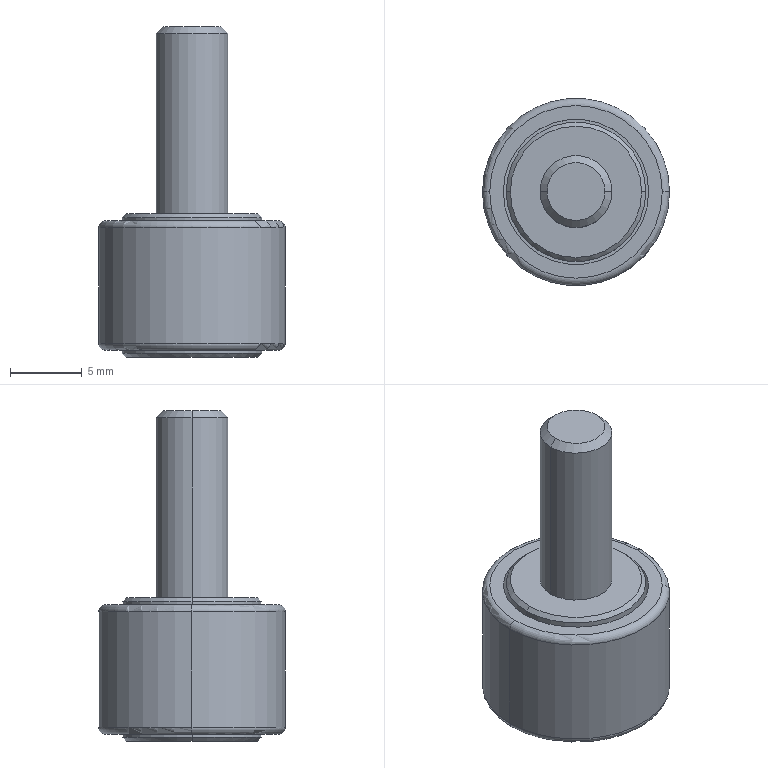Part | NX | features BREP 1 | 1 solid | 36 faces | box 13 x 13 x 23 mm | volume 1465 mm3 | plane 14 | cylinder 12 | cone 6 | torus 4 | commonest cylinder face diameters 9.7 x4 10.1 x4 5 x2 13 x2
STEP:
#1=CARTESIAN_POINT('',(4.567,0.,-23.));
#2=VERTEX_POINT('',#1);
#3=CARTESIAN_POINT('',(-4.567,0.,-23.));
#4=VERTEX_POINT('',#3);
#5=CARTESIAN_POINT('',(0.,0.,-23.));
#6=DIRECTION('',(0.,0.,1.));
#7=DIRECTION('',(1.,0.,0.));
#8=AXIS2_PLACEMENT_3D('',#5,#6,#7);
#9=CIRCLE('',#8,4.567);
#10=EDGE_CURVE('',#2,#4,#9,.T.);
#11=ORIENTED_EDGE('',*,*,#10,.T.);
#12=CARTESIAN_POINT('',(-4.85,0.,-22.717));
#13=VERTEX_POINT('',#12);
#14=CARTESIAN_POINT('',(-4.567,0.,-23.));
#15=DIRECTION('',(-0.7071,0.,0.7071));
#16=VECTOR('',#15,1000.);
#17=LINE('',#14,#16);
#18=EDGE_CURVE('',#4,#13,#17,.T.);
#19=ORIENTED_EDGE('',*,*,#18,.T.);
#20=CARTESIAN_POINT('',(4.85,0.,-22.717));
#21=VERTEX_POINT('',#20);
#22=CARTESIAN_POINT('',(0.,0.,-22.717));
#23=DIRECTION('',(0.,0.,1.));
#24=DIRECTION('',(1.,0.,0.));
#25=AXIS2_PLACEMENT_3D('',#22,#23,#24);
#26=CIRCLE('',#25,4.85);
#27=EDGE_CURVE('',#21,#13,#26,.T.);
#28=ORIENTED_EDGE('',*,*,#27,.F.);
#29=CARTESIAN_POINT('',(4.567,0.,-23.));
#30=DIRECTION('',(0.7071,0.,0.7071));
#31=VECTOR('',#30,1000.);
#32=LINE('',#29,#31);
#33=EDGE_CURVE('',#2,#21,#32,.T.);
#34=ORIENTED_EDGE('',*,*,#33,.F.);
#35=EDGE_LOOP('',(#11,#19,#28,#34));
#36=FACE_BOUND('',#35,.T.);
#37=CARTESIAN_POINT('',(0.,0.,-23.));
#38=DIRECTION('',(0.,0.,1.));
#39=DIRECTION('',(-1.,0.,0.));
#40=AXIS2_PLACEMENT_3D('',#37,#38,#39);
#41=CONICAL_SURFACE('',#40,4.567,0.7854);
#42=ADVANCED_FACE('',(#36),#41,.T.);
#43=ORIENTED_EDGE('',*,*,#27,.T.);
#44=CARTESIAN_POINT('',(-4.85,0.,-21.));
#45=VERTEX_POINT('',#44);
#46=CARTESIAN_POINT('',(-4.85,0.,-23.));
#47=DIRECTION('',(0.,0.,1.));
#48=VECTOR('',#47,1000.);
#49=LINE('',#46,#48);
#50=EDGE_CURVE('',#13,#45,#49,.T.);
#51=ORIENTED_EDGE('',*,*,#50,.T.);
#52=CARTESIAN_POINT('',(4.85,0.,-21.));
#53=VERTEX_POINT('',#52);
#54=CARTESIAN_POINT('',(0.,0.,-21.));
#55=DIRECTION('',(0.,0.,1.));
#56=DIRECTION('',(1.,0.,0.));
#57=AXIS2_PLACEMENT_3D('',#54,#55,#56);
#58=CIRCLE('',#57,4.85);
#59=EDGE_CURVE('',#53,#45,#58,.T.);
#60=ORIENTED_EDGE('',*,*,#59,.F.);
#61=CARTESIAN_POINT('',(4.85,0.,-23.));
#62=DIRECTION('',(0.,0.,1.));
#63=VECTOR('',#62,1000.);
#64=LINE('',#61,#63);
#65=EDGE_CURVE('',#21,#53,#64,.T.);
#66=ORIENTED_EDGE('',*,*,#65,.F.);
#67=EDGE_LOOP('',(#43,#51,#60,#66));
#68=FACE_BOUND('',#67,.T.);
#69=CARTESIAN_POINT('',(0.,0.,-23.));
#70=DIRECTION('',(0.,0.,1.));
#71=DIRECTION('',(-1.,0.,0.));
#72=AXIS2_PLACEMENT_3D('',#69,#70,#71);
#73=CYLINDRICAL_SURFACE('',#72,4.85);
#74=ADVANCED_FACE('',(#68),#73,.T.);
#75=CARTESIAN_POINT('',(-5.05,0.,-22.5));
#76=VERTEX_POINT('',#75);
#77=CARTESIAN_POINT('',(5.05,0.,-22.5));
#78=VERTEX_POINT('',#77);
#79=CARTESIAN_POINT('',(0.,0.,-22.5));
#80=DIRECTION('',(0.,0.,1.));
#81=DIRECTION('',(1.,0.,0.));
#82=AXIS2_PLACEMENT_3D('',#79,#80,#81);
#83=CIRCLE('',#82,5.05);
#84=EDGE_CURVE('',#76,#78,#83,.T.);
#85=ORIENTED_EDGE('',*,*,#84,.F.);
#86=CARTESIAN_POINT('',(-5.05,0.,-21.));
#87=VERTEX_POINT('',#86);
#88=CARTESIAN_POINT('',(-5.05,0.,-23.));
#89=DIRECTION('',(0.,0.,1.));
#90=VECTOR('',#89,1000.);
#91=LINE('',#88,#90);
#92=EDGE_CURVE('',#76,#87,#91,.T.);
#93=ORIENTED_EDGE('',*,*,#92,.T.);
#94=CARTESIAN_POINT('',(5.05,0.,-21.));
#95=VERTEX_POINT('',#94);
#96=CARTESIAN_POINT('',(0.,0.,-21.));
#97=DIRECTION('',(0.,0.,1.));
#98=DIRECTION('',(1.,0.,0.));
#99=AXIS2_PLACEMENT_3D('',#96,#97,#98);
#100=CIRCLE('',#99,5.05);
#101=EDGE_CURVE('',#87,#95,#100,.T.);
#102=ORIENTED_EDGE('',*,*,#101,.T.);
#103=CARTESIAN_POINT('',(5.05,0.,-23.));
#104=DIRECTION('',(0.,0.,1.));
#105=VECTOR('',#104,1000.);
#106=LINE('',#103,#105);
#107=EDGE_CURVE('',#78,#95,#106,.T.);
#108=ORIENTED_EDGE('',*,*,#107,.F.);
#109=EDGE_LOOP('',(#85,#93,#102,#108));
#110=FACE_BOUND('',#109,.T.);
#111=CARTESIAN_POINT('',(0.,0.,-23.));
#112=DIRECTION('',(0.,0.,1.));
#113=DIRECTION('',(-1.,0.,0.));
#114=AXIS2_PLACEMENT_3D('',#111,#112,#113);
#115=CYLINDRICAL_SURFACE('',#114,5.05);
#116=ADVANCED_FACE('',(#110),#115,.F.);
#117=CARTESIAN_POINT('',(6.,0.,-22.5));
#118=VERTEX_POINT('',#117);
#119=CARTESIAN_POINT('',(-6.,0.,-22.5));
#120=VERTEX_POINT('',#119);
#121=CARTESIAN_POINT('',(0.,0.,-22.5));
#122=DIRECTION('',(0.,0.,1.));
#123=DIRECTION('',(1.,0.,0.));
#124=AXIS2_PLACEMENT_3D('',#121,#122,#123);
#125=CIRCLE('',#124,6.);
#126=EDGE_CURVE('',#118,#120,#125,.T.);
#127=ORIENTED_EDGE('',*,*,#126,.T.);
#128=CARTESIAN_POINT('',(-6.5,0.,-22.));
#129=VERTEX_POINT('',#128);
#130=CARTESIAN_POINT('',(-6.,0.,-22.));
#131=DIRECTION('',(0.,1.,0.));
#132=DIRECTION('',(-1.,0.,0.));
#133=AXIS2_PLACEMENT_3D('',#130,#131,#132);
#134=CIRCLE('',#133,0.5);
#135=EDGE_CURVE('',#120,#129,#134,.T.);
#136=ORIENTED_EDGE('',*,*,#135,.T.);
#137=CARTESIAN_POINT('',(6.5,0.,-22.));
#138=VERTEX_POINT('',#137);
#139=CARTESIAN_POINT('',(0.,0.,-22.));
#140=DIRECTION('',(0.,0.,1.));
#141=DIRECTION('',(1.,0.,0.));
#142=AXIS2_PLACEMENT_3D('',#139,#140,#141);
#143=CIRCLE('',#142,6.5);
#144=EDGE_CURVE('',#138,#129,#143,.T.);
#145=ORIENTED_EDGE('',*,*,#144,.F.);
#146=CARTESIAN_POINT('',(6.,0.,-22.));
#147=DIRECTION('',(0.,-1.,0.));
#148=DIRECTION('',(0.,0.,-1.));
#149=AXIS2_PLACEMENT_3D('',#146,#147,#148);
#150=CIRCLE('',#149,0.5);
#151=EDGE_CURVE('',#118,#138,#150,.T.);
#152=ORIENTED_EDGE('',*,*,#151,.F.);
#153=EDGE_LOOP('',(#127,#136,#145,#152));
#154=FACE_BOUND('',#153,.T.);
#155=CARTESIAN_POINT('',(0.,0.,-22.));
#156=DIRECTION('',(0.,0.,1.));
#157=DIRECTION('',(-1.,0.,0.));
#158=AXIS2_PLACEMENT_3D('',#155,#156,#157);
#159=TOROIDAL_SURFACE('',#158,6.,0.5);
#160=ADVANCED_FACE('',(#154),#159,.T.);
#161=ORIENTED_EDGE('',*,*,#144,.T.);
#162=CARTESIAN_POINT('',(-6.5,0.,-14.));
#163=VERTEX_POINT('',#162);
#164=CARTESIAN_POINT('',(-6.5,0.,-23.));
#165=DIRECTION('',(0.,0.,1.));
#166=VECTOR('',#165,1000.);
#167=LINE('',#164,#166);
#168=EDGE_CURVE('',#129,#163,#167,.T.);
#169=ORIENTED_EDGE('',*,*,#168,.T.);
#170=CARTESIAN_POINT('',(6.5,0.,-14.));
#171=VERTEX_POINT('',#170);
#172=CARTESIAN_POINT('',(0.,0.,-14.));
#173=DIRECTION('',(0.,0.,1.));
#174=DIRECTION('',(1.,0.,0.));
#175=AXIS2_PLACEMENT_3D('',#172,#173,#174);
#176=CIRCLE('',#175,6.5);
#177=EDGE_CURVE('',#171,#163,#176,.T.);
#178=ORIENTED_EDGE('',*,*,#177,.F.);
#179=CARTESIAN_POINT('',(6.5,0.,-23.));
#180=DIRECTION('',(0.,0.,1.));
#181=VECTOR('',#180,1000.);
#182=LINE('',#179,#181);
#183=EDGE_CURVE('',#138,#171,#182,.T.);
#184=ORIENTED_EDGE('',*,*,#183,.F.);
#185=EDGE_LOOP('',(#161,#169,#178,#184));
#186=FACE_BOUND('',#185,.T.);
#187=CARTESIAN_POINT('',(0.,0.,-23.));
#188=DIRECTION('',(0.,0.,1.));
#189=DIRECTION('',(-1.,0.,0.));
#190=AXIS2_PLACEMENT_3D('',#187,#188,#189);
#191=CYLINDRICAL_SURFACE('',#190,6.5);
#192=ADVANCED_FACE('',(#186),#191,.T.);
#193=ORIENTED_EDGE('',*,*,#177,.T.);
#194=CARTESIAN_POINT('',(-6.,0.,-13.5));
#195=VERTEX_POINT('',#194);
#196=CARTESIAN_POINT('',(-6.,0.,-14.));
#197=DIRECTION('',(0.,1.,0.));
#198=DIRECTION('',(-1.,0.,0.));
#199=AXIS2_PLACEMENT_3D('',#196,#197,#198);
#200=CIRCLE('',#199,0.5);
#201=EDGE_CURVE('',#163,#195,#200,.T.);
#202=ORIENTED_EDGE('',*,*,#201,.T.);
#203=CARTESIAN_POINT('',(6.,0.,-13.5));
#204=VERTEX_POINT('',#203);
#205=CARTESIAN_POINT('',(0.,0.,-13.5));
#206=DIRECTION('',(0.,0.,1.));
#207=DIRECTION('',(1.,0.,0.));
#208=AXIS2_PLACEMENT_3D('',#205,#206,#207);
#209=CIRCLE('',#208,6.);
#210=EDGE_CURVE('',#204,#195,#209,.T.);
#211=ORIENTED_EDGE('',*,*,#210,.F.);
#212=CARTESIAN_POINT('',(6.,0.,-14.));
#213=DIRECTION('',(0.,-1.,0.));
#214=DIRECTION('',(0.,0.,-1.));
#215=AXIS2_PLACEMENT_3D('',#212,#213,#214);
#216=CIRCLE('',#215,0.5);
#217=EDGE_CURVE('',#171,#204,#216,.T.);
#218=ORIENTED_EDGE('',*,*,#217,.F.);
#219=EDGE_LOOP('',(#193,#202,#211,#218));
#220=FACE_BOUND('',#219,.T.);
#221=CARTESIAN_POINT('',(0.,0.,-14.));
#222=DIRECTION('',(0.,0.,1.));
#223=DIRECTION('',(-1.,0.,0.));
#224=AXIS2_PLACEMENT_3D('',#221,#222,#223);
#225=TOROIDAL_SURFACE('',#224,6.,0.5);
#226=ADVANCED_FACE('',(#220),#225,.T.);
#227=CARTESIAN_POINT('',(-5.05,0.,-15.));
#228=VERTEX_POINT('',#227);
#229=CARTESIAN_POINT('',(5.05,0.,-15.));
#230=VERTEX_POINT('',#229);
#231=CARTESIAN_POINT('',(0.,0.,-15.));
#232=DIRECTION('',(0.,0.,1.));
#233=DIRECTION('',(1.,0.,0.));
#234=AXIS2_PLACEMENT_3D('',#231,#232,#233);
#235=CIRCLE('',#234,5.05);
#236=EDGE_CURVE('',#228,#230,#235,.T.);
#237=ORIENTED_EDGE('',*,*,#236,.F.);
#238=CARTESIAN_POINT('',(-5.05,0.,-13.5));
#239=VERTEX_POINT('',#238);
#240=CARTESIAN_POINT('',(-5.05,0.,-23.));
#241=DIRECTION('',(0.,0.,1.));
#242=VECTOR('',#241,1000.);
#243=LINE('',#240,#242);
#244=EDGE_CURVE('',#228,#239,#243,.T.);
#245=ORIENTED_EDGE('',*,*,#244,.T.);
#246=CARTESIAN_POINT('',(5.05,0.,-13.5));
#247=VERTEX_POINT('',#246);
#248=CARTESIAN_POINT('',(0.,0.,-13.5));
#249=DIRECTION('',(0.,0.,1.));
#250=DIRECTION('',(1.,0.,0.));
#251=AXIS2_PLACEMENT_3D('',#248,#249,#250);
#252=CIRCLE('',#251,5.05);
#253=EDGE_CURVE('',#239,#247,#252,.T.);
#254=ORIENTED_EDGE('',*,*,#253,.T.);
#255=CARTESIAN_POINT('',(5.05,0.,-23.));
#256=DIRECTION('',(0.,0.,1.));
#257=VECTOR('',#256,1000.);
#258=LINE('',#255,#257);
#259=EDGE_CURVE('',#230,#247,#258,.T.);
#260=ORIENTED_EDGE('',*,*,#259,.F.);
#261=EDGE_LOOP('',(#237,#245,#254,#260));
#262=FACE_BOUND('',#261,.T.);
#263=CARTESIAN_POINT('',(0.,0.,-23.));
#264=DIRECTION('',(0.,0.,1.));
#265=DIRECTION('',(-1.,0.,0.));
#266=AXIS2_PLACEMENT_3D('',#263,#264,#265);
#267=CYLINDRICAL_SURFACE('',#266,5.05);
#268=ADVANCED_FACE('',(#262),#267,.F.);
#269=CARTESIAN_POINT('',(4.85,0.,-15.));
#270=VERTEX_POINT('',#269);
#271=CARTESIAN_POINT('',(-4.85,0.,-15.));
#272=VERTEX_POINT('',#271);
#273=CARTESIAN_POINT('',(0.,0.,-15.));
#274=DIRECTION('',(0.,0.,1.));
#275=DIRECTION('',(1.,0.,0.));
#276=AXIS2_PLACEMENT_3D('',#273,#274,#275);
#277=CIRCLE('',#276,4.85);
#278=EDGE_CURVE('',#270,#272,#277,.T.);
#279=ORIENTED_EDGE('',*,*,#278,.T.);
#280=CARTESIAN_POINT('',(-4.85,0.,-13.283));
#281=VERTEX_POINT('',#280);
#282=CARTESIAN_POINT('',(-4.85,0.,-23.));
#283=DIRECTION('',(0.,0.,1.));
#284=VECTOR('',#283,1000.);
#285=LINE('',#282,#284);
#286=EDGE_CURVE('',#272,#281,#285,.T.);
#287=ORIENTED_EDGE('',*,*,#286,.T.);
#288=CARTESIAN_POINT('',(4.85,0.,-13.283));
#289=VERTEX_POINT('',#288);
#290=CARTESIAN_POINT('',(0.,0.,-13.283));
#291=DIRECTION('',(0.,0.,1.));
#292=DIRECTION('',(1.,0.,0.));
#293=AXIS2_PLACEMENT_3D('',#290,#291,#292);
#294=CIRCLE('',#293,4.85);
#295=EDGE_CURVE('',#289,#281,#294,.T.);
#296=ORIENTED_EDGE('',*,*,#295,.F.);
#297=CARTESIAN_POINT('',(4.85,0.,-23.));
#298=DIRECTION('',(0.,0.,1.));
#299=VECTOR('',#298,1000.);
#300=LINE('',#297,#299);
#301=EDGE_CURVE('',#270,#289,#300,.T.);
#302=ORIENTED_EDGE('',*,*,#301,.F.);
#303=EDGE_LOOP('',(#279,#287,#296,#302));
#304=FACE_BOUND('',#303,.T.);
#305=CARTESIAN_POINT('',(0.,0.,-23.));
#306=DIRECTION('',(0.,0.,1.));
#307=DIRECTION('',(-1.,0.,0.));
#308=AXIS2_PLACEMENT_3D('',#305,#306,#307);
#309=CYLINDRICAL_SURFACE('',#308,4.85);
#310=ADVANCED_FACE('',(#304),#309,.T.);
#311=CARTESIAN_POINT('',(4.567,0.,-13.));
#312=VERTEX_POINT('',#311);
#313=CARTESIAN_POINT('',(-4.567,0.,-13.));
#314=VERTEX_POINT('',#313);
#315=CARTESIAN_POINT('',(0.,0.,-13.));
#316=DIRECTION('',(0.,0.,1.));
#317=DIRECTION('',(1.,0.,0.));
#318=AXIS2_PLACEMENT_3D('',#315,#316,#317);
#319=CIRCLE('',#318,4.567);
#320=EDGE_CURVE('',#312,#314,#319,.T.);
#321=ORIENTED_EDGE('',*,*,#320,.F.);
#322=CARTESIAN_POINT('',(4.85,0.,-13.283));
#323=DIRECTION('',(0.7071,0.,-0.7071));
#324=VECTOR('',#323,1000.);
#325=LINE('',#322,#324);
#326=EDGE_CURVE('',#289,#312,#325,.F.);
#327=ORIENTED_EDGE('',*,*,#326,.F.);
#328=ORIENTED_EDGE('',*,*,#295,.T.);
#329=CARTESIAN_POINT('',(-4.85,0.,-13.283));
#330=DIRECTION('',(-0.7071,0.,-0.7071));
#331=VECTOR('',#330,1000.);
#332=LINE('',#329,#331);
#333=EDGE_CURVE('',#281,#314,#332,.F.);
#334=ORIENTED_EDGE('',*,*,#333,.T.);
#335=EDGE_LOOP('',(#321,#327,#328,#334));
#336=FACE_BOUND('',#335,.T.);
#337=CARTESIAN_POINT('',(0.,0.,-13.283));
#338=DIRECTION('',(0.,0.,-1.));
#339=DIRECTION('',(1.,0.,0.));
#340=AXIS2_PLACEMENT_3D('',#337,#338,#339);
#341=CONICAL_SURFACE('',#340,4.85,0.7854);
#342=ADVANCED_FACE('',(#336),#341,.T.);
#343=CARTESIAN_POINT('',(2.5,0.,-13.));
#344=VERTEX_POINT('',#343);
#345=CARTESIAN_POINT('',(-2.5,0.,-13.));
#346=VERTEX_POINT('',#345);
#347=CARTESIAN_POINT('',(0.,0.,-13.));
#348=DIRECTION('',(0.,0.,1.));
#349=DIRECTION('',(1.,0.,0.));
#350=AXIS2_PLACEMENT_3D('',#347,#348,#349);
#351=CIRCLE('',#350,2.5);
#352=EDGE_CURVE('',#344,#346,#351,.T.);
#353=ORIENTED_EDGE('',*,*,#352,.T.);
#354=CARTESIAN_POINT('',(-2.5,0.,-0.4905));
#355=VERTEX_POINT('',#354);
#356=CARTESIAN_POINT('',(-2.5,0.,-23.));
#357=DIRECTION('',(0.,0.,1.));
#358=VECTOR('',#357,1000.);
#359=LINE('',#356,#358);
#360=EDGE_CURVE('',#346,#355,#359,.T.);
#361=ORIENTED_EDGE('',*,*,#360,.T.);
#362=CARTESIAN_POINT('',(2.5,0.,-0.4905));
#363=VERTEX_POINT('',#362);
#364=CARTESIAN_POINT('',(0.,0.,-0.4905));
#365=DIRECTION('',(0.,0.,1.));
#366=DIRECTION('',(1.,0.,0.));
#367=AXIS2_PLACEMENT_3D('',#364,#365,#366);
#368=CIRCLE('',#367,2.5);
#369=EDGE_CURVE('',#363,#355,#368,.T.);
#370=ORIENTED_EDGE('',*,*,#369,.F.);
#371=CARTESIAN_POINT('',(2.5,0.,-23.));
#372=DIRECTION('',(0.,0.,1.));
#373=VECTOR('',#372,1000.);
#374=LINE('',#371,#373);
#375=EDGE_CURVE('',#344,#363,#374,.T.);
#376=ORIENTED_EDGE('',*,*,#375,.F.);
#377=EDGE_LOOP('',(#353,#361,#370,#376));
#378=FACE_BOUND('',#377,.T.);
#379=CARTESIAN_POINT('',(0.,0.,-23.));
#380=DIRECTION('',(0.,0.,1.));
#381=DIRECTION('',(-1.,0.,0.));
#382=AXIS2_PLACEMENT_3D('',#379,#380,#381);
#383=CYLINDRICAL_SURFACE('',#382,2.5);
#384=ADVANCED_FACE('',(#378),#383,.T.);
#385=CARTESIAN_POINT('',(2.01,0.,0.));
#386=VERTEX_POINT('',#385);
#387=CARTESIAN_POINT('',(-2.01,0.,0.));
#388=VERTEX_POINT('',#387);
#389=CARTESIAN_POINT('',(0.,0.,0.));
#390=DIRECTION('',(0.,0.,1.));
#391=DIRECTION('',(1.,0.,0.));
#392=AXIS2_PLACEMENT_3D('',#389,#390,#391);
#393=CIRCLE('',#392,2.01);
#394=EDGE_CURVE('',#386,#388,#393,.T.);
#395=ORIENTED_EDGE('',*,*,#394,.F.);
#396=CARTESIAN_POINT('',(2.5,0.,-0.4905));
#397=DIRECTION('',(0.7071,0.,-0.7071));
#398=VECTOR('',#397,1000.);
#399=LINE('',#396,#398);
#400=EDGE_CURVE('',#363,#386,#399,.F.);
#401=ORIENTED_EDGE('',*,*,#400,.F.);
#402=ORIENTED_EDGE('',*,*,#369,.T.);
#403=CARTESIAN_POINT('',(-2.5,0.,-0.4905));
#404=DIRECTION('',(-0.7071,0.,-0.7071));
#405=VECTOR('',#404,1000.);
#406=LINE('',#403,#405);
#407=EDGE_CURVE('',#355,#388,#406,.F.);
#408=ORIENTED_EDGE('',*,*,#407,.T.);
#409=EDGE_LOOP('',(#395,#401,#402,#408));
#410=FACE_BOUND('',#409,.T.);
#411=CARTESIAN_POINT('',(0.,0.,-0.4905));
#412=DIRECTION('',(0.,0.,-1.));
#413=DIRECTION('',(1.,0.,0.));
#414=AXIS2_PLACEMENT_3D('',#411,#412,#413);
#415=CONICAL_SURFACE('',#414,2.5,0.7854);
#416=ADVANCED_FACE('',(#410),#415,.T.);
#417=ORIENTED_EDGE('',*,*,#10,.F.);
#418=CARTESIAN_POINT('',(0.,0.,-23.));
#419=DIRECTION('',(0.,0.,1.));
#420=DIRECTION('',(1.,0.,0.));
#421=AXIS2_PLACEMENT_3D('',#418,#419,#420);
#422=CIRCLE('',#421,4.567);
#423=EDGE_CURVE('',#4,#2,#422,.T.);
#424=ORIENTED_EDGE('',*,*,#423,.F.);
#425=EDGE_LOOP('',(#417,#424));
#426=FACE_BOUND('',#425,.T.);
#427=CARTESIAN_POINT('',(-1.5,0.866,-23.));
#428=VERTEX_POINT('',#427);
#429=CARTESIAN_POINT('',(-1.5,-0.866,-23.));
#430=VERTEX_POINT('',#429);
#431=CARTESIAN_POINT('',(-1.5,0.866,-23.));
#432=DIRECTION('',(0.,-1.,0.));
#433=VECTOR('',#432,1000.);
#434=LINE('',#431,#433);
#435=EDGE_CURVE('',#428,#430,#434,.T.);
#436=ORIENTED_EDGE('',*,*,#435,.T.);
#437=CARTESIAN_POINT('',(0.,-1.732,-23.));
#438=VERTEX_POINT('',#437);
#439=CARTESIAN_POINT('',(-1.5,-0.866,-23.));
#440=DIRECTION('',(0.866,-0.5,0.));
#441=VECTOR('',#440,1000.);
#442=LINE('',#439,#441);
#443=EDGE_CURVE('',#430,#438,#442,.T.);
#444=ORIENTED_EDGE('',*,*,#443,.T.);
#445=CARTESIAN_POINT('',(1.5,-0.866,-23.));
#446=VERTEX_POINT('',#445);
#447=CARTESIAN_POINT('',(0.,-1.732,-23.));
#448=DIRECTION('',(0.866,0.5,0.));
#449=VECTOR('',#448,1000.);
#450=LINE('',#447,#449);
#451=EDGE_CURVE('',#438,#446,#450,.T.);
#452=ORIENTED_EDGE('',*,*,#451,.T.);
#453=CARTESIAN_POINT('',(1.5,0.866,-23.));
#454=VERTEX_POINT('',#453);
#455=CARTESIAN_POINT('',(1.5,-0.866,-23.));
#456=DIRECTION('',(0.,1.,0.));
#457=VECTOR('',#456,1000.);
#458=LINE('',#455,#457);
#459=EDGE_CURVE('',#446,#454,#458,.T.);
#460=ORIENTED_EDGE('',*,*,#459,.T.);
#461=CARTESIAN_POINT('',(0.,1.732,-23.));
#462=VERTEX_POINT('',#461);
#463=CARTESIAN_POINT('',(1.5,0.866,-23.));
#464=DIRECTION('',(-0.866,0.5,0.));
#465=VECTOR('',#464,1000.);
#466=LINE('',#463,#465);
#467=EDGE_CURVE('',#454,#462,#466,.T.);
#468=ORIENTED_EDGE('',*,*,#467,.T.);
#469=CARTESIAN_POINT('',(0.,1.732,-23.));
#470=DIRECTION('',(-0.866,-0.5,0.));
#471=VECTOR('',#470,1000.);
#472=LINE('',#469,#471);
#473=EDGE_CURVE('',#462,#428,#472,.T.);
#474=ORIENTED_EDGE('',*,*,#473,.T.);
#475=EDGE_LOOP('',(#436,#444,#452,#460,#468,#474));
#476=FACE_BOUND('',#475,.T.);
#477=CARTESIAN_POINT('',(0.,4.567,-23.));
#478=DIRECTION('',(0.,0.,1.));
#479=DIRECTION('',(-1.,0.,0.));
#480=AXIS2_PLACEMENT_3D('',#477,#478,#479);
#481=PLANE('',#480);
#482=ADVANCED_FACE('',(#426,#476),#481,.F.);
#483=CARTESIAN_POINT('',(0.,0.,0.));
#484=DIRECTION('',(0.,0.,1.));
#485=DIRECTION('',(1.,0.,0.));
#486=AXIS2_PLACEMENT_3D('',#483,#484,#485);
#487=CIRCLE('',#486,2.01);
#488=EDGE_CURVE('',#388,#386,#487,.T.);
#489=ORIENTED_EDGE('',*,*,#488,.T.);
#490=ORIENTED_EDGE('',*,*,#394,.T.);
#491=EDGE_LOOP('',(#489,#490));
#492=FACE_BOUND('',#491,.T.);
#493=CARTESIAN_POINT('',(0.,0.,0.));
#494=DIRECTION('',(0.,0.,-1.));
#495=DIRECTION('',(1.,0.,0.));
#496=AXIS2_PLACEMENT_3D('',#493,#494,#495);
#497=PLANE('',#496);
#498=ADVANCED_FACE('',(#492),#497,.F.);
#499=ORIENTED_EDGE('',*,*,#400,.T.);
#500=ORIENTED_EDGE('',*,*,#488,.F.);
#501=ORIENTED_EDGE('',*,*,#407,.F.);
#502=CARTESIAN_POINT('',(0.,0.,-0.4905));
#503=DIRECTION('',(0.,0.,1.));
#504=DIRECTION('',(1.,0.,0.));
#505=AXIS2_PLACEMENT_3D('',#502,#503,#504);
#506=CIRCLE('',#505,2.5);
#507=EDGE_CURVE('',#355,#363,#506,.T.);
#508=ORIENTED_EDGE('',*,*,#507,.T.);
#509=EDGE_LOOP('',(#499,#500,#501,#508));
#510=FACE_BOUND('',#509,.T.);
#511=CARTESIAN_POINT('',(0.,0.,-0.4905));
#512=DIRECTION('',(0.,0.,-1.));
#513=DIRECTION('',(1.,0.,0.));
#514=AXIS2_PLACEMENT_3D('',#511,#512,#513);
#515=CONICAL_SURFACE('',#514,2.5,0.7854);
#516=ADVANCED_FACE('',(#510),#515,.T.);
#517=ORIENTED_EDGE('',*,*,#360,.F.);
#518=CARTESIAN_POINT('',(0.,0.,-13.));
#519=DIRECTION('',(0.,0.,1.));
#520=DIRECTION('',(1.,0.,0.));
#521=AXIS2_PLACEMENT_3D('',#518,#519,#520);
#522=CIRCLE('',#521,2.5);
#523=EDGE_CURVE('',#346,#344,#522,.T.);
#524=ORIENTED_EDGE('',*,*,#523,.T.);
#525=ORIENTED_EDGE('',*,*,#375,.T.);
#526=ORIENTED_EDGE('',*,*,#507,.F.);
#527=EDGE_LOOP('',(#517,#524,#525,#526));
#528=FACE_BOUND('',#527,.T.);
#529=CARTESIAN_POINT('',(0.,0.,-23.));
#530=DIRECTION('',(0.,0.,1.));
#531=DIRECTION('',(-1.,0.,0.));
#532=AXIS2_PLACEMENT_3D('',#529,#530,#531);
#533=CYLINDRICAL_SURFACE('',#532,2.5);
#534=ADVANCED_FACE('',(#528),#533,.T.);
#535=ORIENTED_EDGE('',*,*,#352,.F.);
#536=ORIENTED_EDGE('',*,*,#523,.F.);
#537=EDGE_LOOP('',(#535,#536));
#538=FACE_BOUND('',#537,.T.);
#539=CARTESIAN_POINT('',(0.,0.,-13.));
#540=DIRECTION('',(0.,0.,1.));
#541=DIRECTION('',(1.,0.,0.));
#542=AXIS2_PLACEMENT_3D('',#539,#540,#541);
#543=CIRCLE('',#542,4.567);
#544=EDGE_CURVE('',#314,#312,#543,.T.);
#545=ORIENTED_EDGE('',*,*,#544,.T.);
#546=ORIENTED_EDGE('',*,*,#320,.T.);
#547=EDGE_LOOP('',(#545,#546));
#548=FACE_BOUND('',#547,.T.);
#549=CARTESIAN_POINT('',(0.,2.5,-13.));
#550=DIRECTION('',(0.,0.,-1.));
#551=DIRECTION('',(1.,0.,0.));
#552=AXIS2_PLACEMENT_3D('',#549,#550,#551);
#553=PLANE('',#552);
#554=ADVANCED_FACE('',(#538,#548),#553,.F.);
#555=ORIENTED_EDGE('',*,*,#326,.T.);
#556=ORIENTED_EDGE('',*,*,#544,.F.);
#557=ORIENTED_EDGE('',*,*,#333,.F.);
#558=CARTESIAN_POINT('',(0.,0.,-13.283));
#559=DIRECTION('',(0.,0.,1.));
#560=DIRECTION('',(1.,0.,0.));
#561=AXIS2_PLACEMENT_3D('',#558,#559,#560);
#562=CIRCLE('',#561,4.85);
#563=EDGE_CURVE('',#281,#289,#562,.T.);
#564=ORIENTED_EDGE('',*,*,#563,.T.);
#565=EDGE_LOOP('',(#555,#556,#557,#564));
#566=FACE_BOUND('',#565,.T.);
#567=CARTESIAN_POINT('',(0.,0.,-13.283));
#568=DIRECTION('',(0.,0.,-1.));
#569=DIRECTION('',(1.,0.,0.));
#570=AXIS2_PLACEMENT_3D('',#567,#568,#569);
#571=CONICAL_SURFACE('',#570,4.85,0.7854);
#572=ADVANCED_FACE('',(#566),#571,.T.);
#573=ORIENTED_EDGE('',*,*,#286,.F.);
#574=CARTESIAN_POINT('',(0.,0.,-15.));
#575=DIRECTION('',(0.,0.,1.));
#576=DIRECTION('',(1.,0.,0.));
#577=AXIS2_PLACEMENT_3D('',#574,#575,#576);
#578=CIRCLE('',#577,4.85);
#579=EDGE_CURVE('',#272,#270,#578,.T.);
#580=ORIENTED_EDGE('',*,*,#579,.T.);
#581=ORIENTED_EDGE('',*,*,#301,.T.);
#582=ORIENTED_EDGE('',*,*,#563,.F.);
#583=EDGE_LOOP('',(#573,#580,#581,#582));
#584=FACE_BOUND('',#583,.T.);
#585=CARTESIAN_POINT('',(0.,0.,-23.));
#586=DIRECTION('',(0.,0.,1.));
#587=DIRECTION('',(-1.,0.,0.));
#588=AXIS2_PLACEMENT_3D('',#585,#586,#587);
#589=CYLINDRICAL_SURFACE('',#588,4.85);
#590=ADVANCED_FACE('',(#584),#589,.T.);
#591=ORIENTED_EDGE('',*,*,#278,.F.);
#592=ORIENTED_EDGE('',*,*,#579,.F.);
#593=EDGE_LOOP('',(#591,#592));
#594=FACE_BOUND('',#593,.T.);
#595=CARTESIAN_POINT('',(0.,0.,-15.));
#596=DIRECTION('',(0.,0.,1.));
#597=DIRECTION('',(1.,0.,0.));
#598=AXIS2_PLACEMENT_3D('',#595,#596,#597);
#599=CIRCLE('',#598,5.05);
#600=EDGE_CURVE('',#230,#228,#599,.T.);
#601=ORIENTED_EDGE('',*,*,#600,.T.);
#602=ORIENTED_EDGE('',*,*,#236,.T.);
#603=EDGE_LOOP('',(#601,#602));
#604=FACE_BOUND('',#603,.T.);
#605=CARTESIAN_POINT('',(0.,4.85,-15.));
#606=DIRECTION('',(0.,0.,-1.));
#607=DIRECTION('',(1.,0.,0.));
#608=AXIS2_PLACEMENT_3D('',#605,#606,#607);
#609=PLANE('',#608);
#610=ADVANCED_FACE('',(#594,#604),#609,.F.);
#611=ORIENTED_EDGE('',*,*,#244,.F.);
#612=ORIENTED_EDGE('',*,*,#600,.F.);
#613=ORIENTED_EDGE('',*,*,#259,.T.);
#614=CARTESIAN_POINT('',(0.,0.,-13.5));
#615=DIRECTION('',(0.,0.,1.));
#616=DIRECTION('',(1.,0.,0.));
#617=AXIS2_PLACEMENT_3D('',#614,#615,#616);
#618=CIRCLE('',#617,5.05);
#619=EDGE_CURVE('',#247,#239,#618,.T.);
#620=ORIENTED_EDGE('',*,*,#619,.T.);
#621=EDGE_LOOP('',(#611,#612,#613,#620));
#622=FACE_BOUND('',#621,.T.);
#623=CARTESIAN_POINT('',(0.,0.,-23.));
#624=DIRECTION('',(0.,0.,1.));
#625=DIRECTION('',(-1.,0.,0.));
#626=AXIS2_PLACEMENT_3D('',#623,#624,#625);
#627=CYLINDRICAL_SURFACE('',#626,5.05);
#628=ADVANCED_FACE('',(#622),#627,.F.);
#629=ORIENTED_EDGE('',*,*,#619,.F.);
#630=ORIENTED_EDGE('',*,*,#253,.F.);
#631=EDGE_LOOP('',(#629,#630));
#632=FACE_BOUND('',#631,.T.);
#633=ORIENTED_EDGE('',*,*,#210,.T.);
#634=CARTESIAN_POINT('',(0.,0.,-13.5));
#635=DIRECTION('',(0.,0.,1.));
#636=DIRECTION('',(1.,0.,0.));
#637=AXIS2_PLACEMENT_3D('',#634,#635,#636);
#638=CIRCLE('',#637,6.);
#639=EDGE_CURVE('',#195,#204,#638,.T.);
#640=ORIENTED_EDGE('',*,*,#639,.T.);
#641=EDGE_LOOP('',(#633,#640));
#642=FACE_BOUND('',#641,.T.);
#643=CARTESIAN_POINT('',(0.,5.05,-13.5));
#644=DIRECTION('',(0.,0.,-1.));
#645=DIRECTION('',(1.,0.,0.));
#646=AXIS2_PLACEMENT_3D('',#643,#644,#645);
#647=PLANE('',#646);
#648=ADVANCED_FACE('',(#632,#642),#647,.F.);
#649=ORIENTED_EDGE('',*,*,#201,.F.);
#650=CARTESIAN_POINT('',(0.,0.,-14.));
#651=DIRECTION('',(0.,0.,1.));
#652=DIRECTION('',(1.,0.,0.));
#653=AXIS2_PLACEMENT_3D('',#650,#651,#652);
#654=CIRCLE('',#653,6.5);
#655=EDGE_CURVE('',#163,#171,#654,.T.);
#656=ORIENTED_EDGE('',*,*,#655,.T.);
#657=ORIENTED_EDGE('',*,*,#217,.T.);
#658=ORIENTED_EDGE('',*,*,#639,.F.);
#659=EDGE_LOOP('',(#649,#656,#657,#658));
#660=FACE_BOUND('',#659,.T.);
#661=CARTESIAN_POINT('',(0.,0.,-14.));
#662=DIRECTION('',(0.,0.,1.));
#663=DIRECTION('',(-1.,0.,0.));
#664=AXIS2_PLACEMENT_3D('',#661,#662,#663);
#665=TOROIDAL_SURFACE('',#664,6.,0.5);
#666=ADVANCED_FACE('',(#660),#665,.T.);
#667=ORIENTED_EDGE('',*,*,#168,.F.);
#668=CARTESIAN_POINT('',(0.,0.,-22.));
#669=DIRECTION('',(0.,0.,1.));
#670=DIRECTION('',(1.,0.,0.));
#671=AXIS2_PLACEMENT_3D('',#668,#669,#670);
#672=CIRCLE('',#671,6.5);
#673=EDGE_CURVE('',#129,#138,#672,.T.);
#674=ORIENTED_EDGE('',*,*,#673,.T.);
#675=ORIENTED_EDGE('',*,*,#183,.T.);
#676=ORIENTED_EDGE('',*,*,#655,.F.);
#677=EDGE_LOOP('',(#667,#674,#675,#676));
#678=FACE_BOUND('',#677,.T.);
#679=CARTESIAN_POINT('',(0.,0.,-23.));
#680=DIRECTION('',(0.,0.,1.));
#681=DIRECTION('',(-1.,0.,0.));
#682=AXIS2_PLACEMENT_3D('',#679,#680,#681);
#683=CYLINDRICAL_SURFACE('',#682,6.5);
#684=ADVANCED_FACE('',(#678),#683,.T.);
#685=ORIENTED_EDGE('',*,*,#135,.F.);
#686=CARTESIAN_POINT('',(0.,0.,-22.5));
#687=DIRECTION('',(0.,0.,1.));
#688=DIRECTION('',(1.,0.,0.));
#689=AXIS2_PLACEMENT_3D('',#686,#687,#688);
#690=CIRCLE('',#689,6.);
#691=EDGE_CURVE('',#120,#118,#690,.T.);
#692=ORIENTED_EDGE('',*,*,#691,.T.);
#693=ORIENTED_EDGE('',*,*,#151,.T.);
#694=ORIENTED_EDGE('',*,*,#673,.F.);
#695=EDGE_LOOP('',(#685,#692,#693,#694));
#696=FACE_BOUND('',#695,.T.);
#697=CARTESIAN_POINT('',(0.,0.,-22.));
#698=DIRECTION('',(0.,0.,1.));
#699=DIRECTION('',(-1.,0.,0.));
#700=AXIS2_PLACEMENT_3D('',#697,#698,#699);
#701=TOROIDAL_SURFACE('',#700,6.,0.5);
#702=ADVANCED_FACE('',(#696),#701,.T.);
#703=ORIENTED_EDGE('',*,*,#126,.F.);
#704=ORIENTED_EDGE('',*,*,#691,.F.);
#705=EDGE_LOOP('',(#703,#704));
#706=FACE_BOUND('',#705,.T.);
#707=CARTESIAN_POINT('',(0.,0.,-22.5));
#708=DIRECTION('',(0.,0.,1.));
#709=DIRECTION('',(1.,0.,0.));
#710=AXIS2_PLACEMENT_3D('',#707,#708,#709);
#711=CIRCLE('',#710,5.05);
#712=EDGE_CURVE('',#78,#76,#711,.T.);
#713=ORIENTED_EDGE('',*,*,#712,.T.);
#714=ORIENTED_EDGE('',*,*,#84,.T.);
#715=EDGE_LOOP('',(#713,#714));
#716=FACE_BOUND('',#715,.T.);
#717=CARTESIAN_POINT('',(0.,6.,-22.5));
#718=DIRECTION('',(0.,0.,1.));
#719=DIRECTION('',(-1.,0.,0.));
#720=AXIS2_PLACEMENT_3D('',#717,#718,#719);
#721=PLANE('',#720);
#722=ADVANCED_FACE('',(#706,#716),#721,.F.);
#723=ORIENTED_EDGE('',*,*,#92,.F.);
#724=ORIENTED_EDGE('',*,*,#712,.F.);
#725=ORIENTED_EDGE('',*,*,#107,.T.);
#726=CARTESIAN_POINT('',(0.,0.,-21.));
#727=DIRECTION('',(0.,0.,1.));
#728=DIRECTION('',(1.,0.,0.));
#729=AXIS2_PLACEMENT_3D('',#726,#727,#728);
#730=CIRCLE('',#729,5.05);
#731=EDGE_CURVE('',#95,#87,#730,.T.);
#732=ORIENTED_EDGE('',*,*,#731,.T.);
#733=EDGE_LOOP('',(#723,#724,#725,#732));
#734=FACE_BOUND('',#733,.T.);
#735=CARTESIAN_POINT('',(0.,0.,-23.));
#736=DIRECTION('',(0.,0.,1.));
#737=DIRECTION('',(-1.,0.,0.));
#738=AXIS2_PLACEMENT_3D('',#735,#736,#737);
#739=CYLINDRICAL_SURFACE('',#738,5.05);
#740=ADVANCED_FACE('',(#734),#739,.F.);
#741=ORIENTED_EDGE('',*,*,#731,.F.);
#742=ORIENTED_EDGE('',*,*,#101,.F.);
#743=EDGE_LOOP('',(#741,#742));
#744=FACE_BOUND('',#743,.T.);
#745=ORIENTED_EDGE('',*,*,#59,.T.);
#746=CARTESIAN_POINT('',(0.,0.,-21.));
#747=DIRECTION('',(0.,0.,1.));
#748=DIRECTION('',(1.,0.,0.));
#749=AXIS2_PLACEMENT_3D('',#746,#747,#748);
#750=CIRCLE('',#749,4.85);
#751=EDGE_CURVE('',#45,#53,#750,.T.);
#752=ORIENTED_EDGE('',*,*,#751,.T.);
#753=EDGE_LOOP('',(#745,#752));
#754=FACE_BOUND('',#753,.T.);
#755=CARTESIAN_POINT('',(0.,5.05,-21.));
#756=DIRECTION('',(0.,0.,1.));
#757=DIRECTION('',(-1.,0.,0.));
#758=AXIS2_PLACEMENT_3D('',#755,#756,#757);
#759=PLANE('',#758);
#760=ADVANCED_FACE('',(#744,#754),#759,.F.);
#761=ORIENTED_EDGE('',*,*,#50,.F.);
#762=CARTESIAN_POINT('',(0.,0.,-22.717));
#763=DIRECTION('',(0.,0.,1.));
#764=DIRECTION('',(1.,0.,0.));
#765=AXIS2_PLACEMENT_3D('',#762,#763,#764);
#766=CIRCLE('',#765,4.85);
#767=EDGE_CURVE('',#13,#21,#766,.T.);
#768=ORIENTED_EDGE('',*,*,#767,.T.);
#769=ORIENTED_EDGE('',*,*,#65,.T.);
#770=ORIENTED_EDGE('',*,*,#751,.F.);
#771=EDGE_LOOP('',(#761,#768,#769,#770));
#772=FACE_BOUND('',#771,.T.);
#773=CARTESIAN_POINT('',(0.,0.,-23.));
#774=DIRECTION('',(0.,0.,1.));
#775=DIRECTION('',(-1.,0.,0.));
#776=AXIS2_PLACEMENT_3D('',#773,#774,#775);
#777=CYLINDRICAL_SURFACE('',#776,4.85);
#778=ADVANCED_FACE('',(#772),#777,.T.);
#779=ORIENTED_EDGE('',*,*,#18,.F.);
#780=ORIENTED_EDGE('',*,*,#423,.T.);
#781=ORIENTED_EDGE('',*,*,#33,.T.);
#782=ORIENTED_EDGE('',*,*,#767,.F.);
#783=EDGE_LOOP('',(#779,#780,#781,#782));
#784=FACE_BOUND('',#783,.T.);
#785=CARTESIAN_POINT('',(0.,0.,-23.));
#786=DIRECTION('',(0.,0.,1.));
#787=DIRECTION('',(-1.,0.,0.));
#788=AXIS2_PLACEMENT_3D('',#785,#786,#787);
#789=CONICAL_SURFACE('',#788,4.567,0.7854);
#790=ADVANCED_FACE('',(#784),#789,.T.);
#791=ORIENTED_EDGE('',*,*,#435,.F.);
#792=CARTESIAN_POINT('',(-1.5,0.866,-19.));
#793=VERTEX_POINT('',#792);
#794=CARTESIAN_POINT('',(-1.5,0.866,-19.));
#795=DIRECTION('',(0.,0.,-1.));
#796=VECTOR('',#795,1000.);
#797=LINE('',#794,#796);
#798=EDGE_CURVE('',#793,#428,#797,.T.);
#799=ORIENTED_EDGE('',*,*,#798,.F.);
#800=CARTESIAN_POINT('',(-1.5,-0.866,-19.));
#801=VERTEX_POINT('',#800);
#802=CARTESIAN_POINT('',(-1.5,0.866,-19.));
#803=DIRECTION('',(0.,-1.,0.));
#804=VECTOR('',#803,1000.);
#805=LINE('',#802,#804);
#806=EDGE_CURVE('',#793,#801,#805,.T.);
#807=ORIENTED_EDGE('',*,*,#806,.T.);
#808=CARTESIAN_POINT('',(-1.5,-0.866,-19.));
#809=DIRECTION('',(0.,0.,-1.));
#810=VECTOR('',#809,1000.);
#811=LINE('',#808,#810);
#812=EDGE_CURVE('',#801,#430,#811,.T.);
#813=ORIENTED_EDGE('',*,*,#812,.T.);
#814=EDGE_LOOP('',(#791,#799,#807,#813));
#815=FACE_BOUND('',#814,.T.);
#816=CARTESIAN_POINT('',(-1.5,0.866,-19.));
#817=DIRECTION('',(1.,0.,0.));
#818=DIRECTION('',(0.,0.,1.));
#819=AXIS2_PLACEMENT_3D('',#816,#817,#818);
#820=PLANE('',#819);
#821=ADVANCED_FACE('',(#815),#820,.T.);
#822=ORIENTED_EDGE('',*,*,#443,.F.);
#823=ORIENTED_EDGE('',*,*,#812,.F.);
#824=CARTESIAN_POINT('',(0.,-1.732,-19.));
#825=VERTEX_POINT('',#824);
#826=CARTESIAN_POINT('',(-1.5,-0.866,-19.));
#827=DIRECTION('',(0.866,-0.5,0.));
#828=VECTOR('',#827,1000.);
#829=LINE('',#826,#828);
#830=EDGE_CURVE('',#801,#825,#829,.T.);
#831=ORIENTED_EDGE('',*,*,#830,.T.);
#832=CARTESIAN_POINT('',(0.,-1.732,-19.));
#833=DIRECTION('',(0.,0.,-1.));
#834=VECTOR('',#833,1000.);
#835=LINE('',#832,#834);
#836=EDGE_CURVE('',#825,#438,#835,.T.);
#837=ORIENTED_EDGE('',*,*,#836,.T.);
#838=EDGE_LOOP('',(#822,#823,#831,#837));
#839=FACE_BOUND('',#838,.T.);
#840=CARTESIAN_POINT('',(-1.5,-0.866,-19.));
#841=DIRECTION('',(0.5,0.866,0.));
#842=DIRECTION('',(0.866,-0.5,0.));
#843=AXIS2_PLACEMENT_3D('',#840,#841,#842);
#844=PLANE('',#843);
#845=ADVANCED_FACE('',(#839),#844,.T.);
#846=ORIENTED_EDGE('',*,*,#451,.F.);
#847=ORIENTED_EDGE('',*,*,#836,.F.);
#848=CARTESIAN_POINT('',(1.5,-0.866,-19.));
#849=VERTEX_POINT('',#848);
#850=CARTESIAN_POINT('',(0.,-1.732,-19.));
#851=DIRECTION('',(0.866,0.5,0.));
#852=VECTOR('',#851,1000.);
#853=LINE('',#850,#852);
#854=EDGE_CURVE('',#825,#849,#853,.T.);
#855=ORIENTED_EDGE('',*,*,#854,.T.);
#856=CARTESIAN_POINT('',(1.5,-0.866,-19.));
#857=DIRECTION('',(0.,0.,-1.));
#858=VECTOR('',#857,1000.);
#859=LINE('',#856,#858);
#860=EDGE_CURVE('',#849,#446,#859,.T.);
#861=ORIENTED_EDGE('',*,*,#860,.T.);
#862=EDGE_LOOP('',(#846,#847,#855,#861));
#863=FACE_BOUND('',#862,.T.);
#864=CARTESIAN_POINT('',(0.,-1.732,-19.));
#865=DIRECTION('',(-0.5,0.866,0.));
#866=DIRECTION('',(0.866,0.5,0.));
#867=AXIS2_PLACEMENT_3D('',#864,#865,#866);
#868=PLANE('',#867);
#869=ADVANCED_FACE('',(#863),#868,.T.);
#870=ORIENTED_EDGE('',*,*,#459,.F.);
#871=ORIENTED_EDGE('',*,*,#860,.F.);
#872=CARTESIAN_POINT('',(1.5,0.866,-19.));
#873=VERTEX_POINT('',#872);
#874=CARTESIAN_POINT('',(1.5,-0.866,-19.));
#875=DIRECTION('',(0.,1.,0.));
#876=VECTOR('',#875,1000.);
#877=LINE('',#874,#876);
#878=EDGE_CURVE('',#849,#873,#877,.T.);
#879=ORIENTED_EDGE('',*,*,#878,.T.);
#880=CARTESIAN_POINT('',(1.5,0.866,-19.));
#881=DIRECTION('',(0.,0.,-1.));
#882=VECTOR('',#881,1000.);
#883=LINE('',#880,#882);
#884=EDGE_CURVE('',#873,#454,#883,.T.);
#885=ORIENTED_EDGE('',*,*,#884,.T.);
#886=EDGE_LOOP('',(#870,#871,#879,#885));
#887=FACE_BOUND('',#886,.T.);
#888=CARTESIAN_POINT('',(1.5,-0.866,-19.));
#889=DIRECTION('',(-1.,0.,0.));
#890=DIRECTION('',(0.,0.,-1.));
#891=AXIS2_PLACEMENT_3D('',#888,#889,#890);
#892=PLANE('',#891);
#893=ADVANCED_FACE('',(#887),#892,.T.);
#894=ORIENTED_EDGE('',*,*,#467,.F.);
#895=ORIENTED_EDGE('',*,*,#884,.F.);
#896=CARTESIAN_POINT('',(0.,1.732,-19.));
#897=VERTEX_POINT('',#896);
#898=CARTESIAN_POINT('',(1.5,0.866,-19.));
#899=DIRECTION('',(-0.866,0.5,0.));
#900=VECTOR('',#899,1000.);
#901=LINE('',#898,#900);
#902=EDGE_CURVE('',#873,#897,#901,.T.);
#903=ORIENTED_EDGE('',*,*,#902,.T.);
#904=CARTESIAN_POINT('',(0.,1.732,-19.));
#905=DIRECTION('',(0.,0.,-1.));
#906=VECTOR('',#905,1000.);
#907=LINE('',#904,#906);
#908=EDGE_CURVE('',#897,#462,#907,.T.);
#909=ORIENTED_EDGE('',*,*,#908,.T.);
#910=EDGE_LOOP('',(#894,#895,#903,#909));
#911=FACE_BOUND('',#910,.T.);
#912=CARTESIAN_POINT('',(1.5,0.866,-19.));
#913=DIRECTION('',(-0.5,-0.866,0.));
#914=DIRECTION('',(-0.866,0.5,0.));
#915=AXIS2_PLACEMENT_3D('',#912,#913,#914);
#916=PLANE('',#915);
#917=ADVANCED_FACE('',(#911),#916,.T.);
#918=ORIENTED_EDGE('',*,*,#473,.F.);
#919=ORIENTED_EDGE('',*,*,#908,.F.);
#920=CARTESIAN_POINT('',(0.,1.732,-19.));
#921=DIRECTION('',(-0.866,-0.5,0.));
#922=VECTOR('',#921,1000.);
#923=LINE('',#920,#922);
#924=EDGE_CURVE('',#897,#793,#923,.T.);
#925=ORIENTED_EDGE('',*,*,#924,.T.);
#926=ORIENTED_EDGE('',*,*,#798,.T.);
#927=EDGE_LOOP('',(#918,#919,#925,#926));
#928=FACE_BOUND('',#927,.T.);
#929=CARTESIAN_POINT('',(0.,1.732,-19.));
#930=DIRECTION('',(0.5,-0.866,0.));
#931=DIRECTION('',(-0.866,-0.5,0.));
#932=AXIS2_PLACEMENT_3D('',#929,#930,#931);
#933=PLANE('',#932);
#934=ADVANCED_FACE('',(#928),#933,.T.);
#935=ORIENTED_EDGE('',*,*,#806,.F.);
#936=ORIENTED_EDGE('',*,*,#924,.F.);
#937=ORIENTED_EDGE('',*,*,#902,.F.);
#938=ORIENTED_EDGE('',*,*,#878,.F.);
#939=ORIENTED_EDGE('',*,*,#854,.F.);
#940=ORIENTED_EDGE('',*,*,#830,.F.);
#941=EDGE_LOOP('',(#935,#936,#937,#938,#939,#940));
#942=FACE_BOUND('',#941,.T.);
#943=CARTESIAN_POINT('',(0.,0.,-19.));
#944=DIRECTION('',(0.,0.,1.));
#945=DIRECTION('',(-1.,0.,0.));
#946=AXIS2_PLACEMENT_3D('',#943,#944,#945);
#947=PLANE('',#946);
#948=ADVANCED_FACE('',(#942),#947,.F.);
#949=CLOSED_SHELL('',(#42,#74,#116,#160,#192,#226,#268,#310,#342,#384,#416,#482,#498,#516,#534,#554,#572,#590,#610,#628,#648,#666,#684,#702,#722,#740,#760,#778,#790,#821,#845,#869,#893,#917,#934,#948));
#950=MANIFOLD_SOLID_BREP('',#949);
#951=(LENGTH_UNIT()NAMED_UNIT(*)SI_UNIT(.MILLI.,.METRE.));
#952=UNCERTAINTY_MEASURE_WITH_UNIT(LENGTH_MEASURE(0.00001),#951,'','');
#953=(NAMED_UNIT(*)PLANE_ANGLE_UNIT()SI_UNIT($,.RADIAN.));
#954=(NAMED_UNIT(*)SI_UNIT($,.STERADIAN.)SOLID_ANGLE_UNIT());
#955=(GEOMETRIC_REPRESENTATION_CONTEXT(3)GLOBAL_UNCERTAINTY_ASSIGNED_CONTEXT((#952))GLOBAL_UNIT_ASSIGNED_CONTEXT((#951,#953,#954))REPRESENTATION_CONTEXT('',''));
#956=ADVANCED_BREP_SHAPE_REPRESENTATION('',(#950),#955);